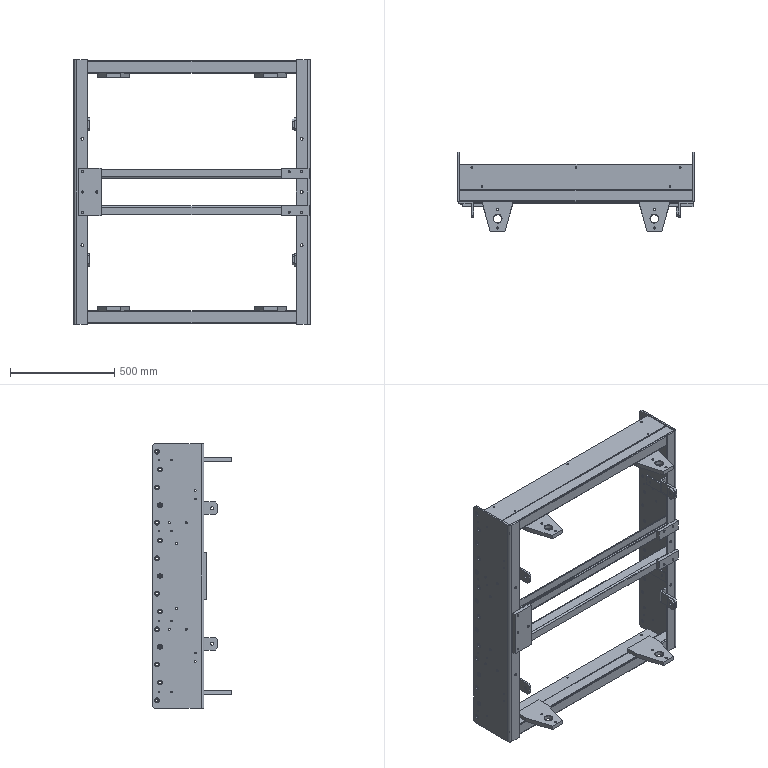Part | SolidWorks | features CompositeCurve 3 | 25 solids | 570 faces | box 1132 x 377 x 1270 mm | volume 14549074 mm3 | cylinder 282 | plane 212 | cone 76 | commonest cylinder face diameters 10.2 x64 12.5 x60 6.8 x48 8.5 x24 10 x16 13 x16